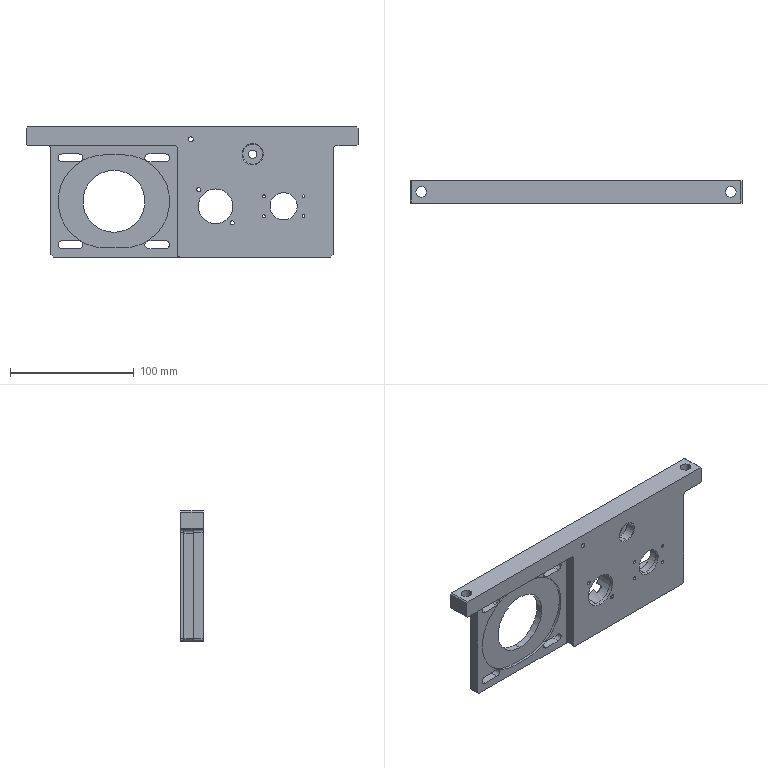Part | STEP file | PN_0001 Lead Screw Support Block (Right) | 1 solid | 121 faces | box 268 x 18 x 105 mm | volume 283725 mm3 | cylinder 68 | plane 42 | cone 11 | commonest cylinder face diameters 2.4 x8 4 x8 6.5 x8 4.2 x6 9 x6 75 x6